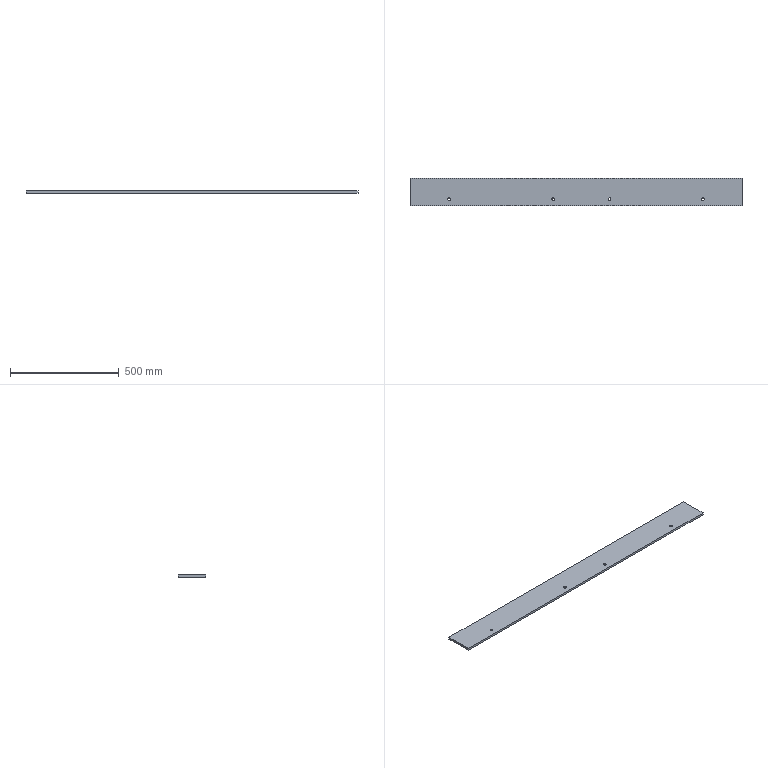Part | NX | features BREP 1 | 1 solid | 14 faces | box 1530 x 126 x 10 mm | volume 1923276 mm3 | cylinder 8 | plane 6 | commonest cylinder face diameters 12 x8
STEP:
#1=CARTESIAN_POINT('',(-591.,-33.,-5.));
#2=VERTEX_POINT('',#1);
#3=CARTESIAN_POINT('',(-579.,-33.,-5.));
#4=VERTEX_POINT('',#3);
#5=CARTESIAN_POINT('',(-585.,-33.,-5.));
#6=DIRECTION('',(0.,0.,-1.));
#7=DIRECTION('',(1.,0.,0.));
#8=AXIS2_PLACEMENT_3D('',#5,#6,#7);
#9=CIRCLE('',#8,6.);
#10=EDGE_CURVE('',#2,#4,#9,.T.);
#11=ORIENTED_EDGE('',*,*,#10,.T.);
#12=CARTESIAN_POINT('',(-579.,-33.,5.));
#13=VERTEX_POINT('',#12);
#14=CARTESIAN_POINT('',(-579.,-33.,-5.));
#15=DIRECTION('',(0.,0.,1.));
#16=VECTOR('',#15,1000.);
#17=LINE('',#14,#16);
#18=EDGE_CURVE('',#13,#4,#17,.F.);
#19=ORIENTED_EDGE('',*,*,#18,.F.);
#20=CARTESIAN_POINT('',(-591.,-33.,5.));
#21=VERTEX_POINT('',#20);
#22=CARTESIAN_POINT('',(-585.,-33.,5.));
#23=DIRECTION('',(0.,0.,-1.));
#24=DIRECTION('',(1.,0.,0.));
#25=AXIS2_PLACEMENT_3D('',#22,#23,#24);
#26=CIRCLE('',#25,6.);
#27=EDGE_CURVE('',#21,#13,#26,.T.);
#28=ORIENTED_EDGE('',*,*,#27,.F.);
#29=CARTESIAN_POINT('',(-591.,-33.,-5.));
#30=DIRECTION('',(0.,0.,1.));
#31=VECTOR('',#30,1000.);
#32=LINE('',#29,#31);
#33=EDGE_CURVE('',#21,#2,#32,.F.);
#34=ORIENTED_EDGE('',*,*,#33,.T.);
#35=EDGE_LOOP('',(#11,#19,#28,#34));
#36=FACE_BOUND('',#35,.T.);
#37=CARTESIAN_POINT('',(-585.,-33.,-5.));
#38=DIRECTION('',(0.,0.,1.));
#39=DIRECTION('',(1.,0.,0.));
#40=AXIS2_PLACEMENT_3D('',#37,#38,#39);
#41=CYLINDRICAL_SURFACE('',#40,6.);
#42=ADVANCED_FACE('',(#36),#41,.F.);
#43=CARTESIAN_POINT('',(-111.,-33.,-5.));
#44=VERTEX_POINT('',#43);
#45=CARTESIAN_POINT('',(-99.,-33.,-5.));
#46=VERTEX_POINT('',#45);
#47=CARTESIAN_POINT('',(-105.,-33.,-5.));
#48=DIRECTION('',(0.,0.,-1.));
#49=DIRECTION('',(1.,0.,0.));
#50=AXIS2_PLACEMENT_3D('',#47,#48,#49);
#51=CIRCLE('',#50,6.);
#52=EDGE_CURVE('',#44,#46,#51,.T.);
#53=ORIENTED_EDGE('',*,*,#52,.T.);
#54=CARTESIAN_POINT('',(-99.,-33.,5.));
#55=VERTEX_POINT('',#54);
#56=CARTESIAN_POINT('',(-99.,-33.,-5.));
#57=DIRECTION('',(0.,0.,1.));
#58=VECTOR('',#57,1000.);
#59=LINE('',#56,#58);
#60=EDGE_CURVE('',#55,#46,#59,.F.);
#61=ORIENTED_EDGE('',*,*,#60,.F.);
#62=CARTESIAN_POINT('',(-111.,-33.,5.));
#63=VERTEX_POINT('',#62);
#64=CARTESIAN_POINT('',(-105.,-33.,5.));
#65=DIRECTION('',(0.,0.,-1.));
#66=DIRECTION('',(1.,0.,0.));
#67=AXIS2_PLACEMENT_3D('',#64,#65,#66);
#68=CIRCLE('',#67,6.);
#69=EDGE_CURVE('',#63,#55,#68,.T.);
#70=ORIENTED_EDGE('',*,*,#69,.F.);
#71=CARTESIAN_POINT('',(-111.,-33.,-5.));
#72=DIRECTION('',(0.,0.,1.));
#73=VECTOR('',#72,1000.);
#74=LINE('',#71,#73);
#75=EDGE_CURVE('',#63,#44,#74,.F.);
#76=ORIENTED_EDGE('',*,*,#75,.T.);
#77=EDGE_LOOP('',(#53,#61,#70,#76));
#78=FACE_BOUND('',#77,.T.);
#79=CARTESIAN_POINT('',(-105.,-33.,-5.));
#80=DIRECTION('',(0.,0.,1.));
#81=DIRECTION('',(1.,0.,0.));
#82=AXIS2_PLACEMENT_3D('',#79,#80,#81);
#83=CYLINDRICAL_SURFACE('',#82,6.);
#84=ADVANCED_FACE('',(#78),#83,.F.);
#85=CARTESIAN_POINT('',(149.,-33.,-5.));
#86=VERTEX_POINT('',#85);
#87=CARTESIAN_POINT('',(161.,-33.,-5.));
#88=VERTEX_POINT('',#87);
#89=CARTESIAN_POINT('',(155.,-33.,-5.));
#90=DIRECTION('',(0.,0.,-1.));
#91=DIRECTION('',(-1.,0.,0.));
#92=AXIS2_PLACEMENT_3D('',#89,#90,#91);
#93=CIRCLE('',#92,6.);
#94=EDGE_CURVE('',#86,#88,#93,.T.);
#95=ORIENTED_EDGE('',*,*,#94,.T.);
#96=CARTESIAN_POINT('',(161.,-33.,5.));
#97=VERTEX_POINT('',#96);
#98=CARTESIAN_POINT('',(161.,-33.,-5.));
#99=DIRECTION('',(0.,0.,1.));
#100=VECTOR('',#99,1000.);
#101=LINE('',#98,#100);
#102=EDGE_CURVE('',#97,#88,#101,.F.);
#103=ORIENTED_EDGE('',*,*,#102,.F.);
#104=CARTESIAN_POINT('',(149.,-33.,5.));
#105=VERTEX_POINT('',#104);
#106=CARTESIAN_POINT('',(155.,-33.,5.));
#107=DIRECTION('',(0.,0.,-1.));
#108=DIRECTION('',(-1.,0.,0.));
#109=AXIS2_PLACEMENT_3D('',#106,#107,#108);
#110=CIRCLE('',#109,6.);
#111=EDGE_CURVE('',#105,#97,#110,.T.);
#112=ORIENTED_EDGE('',*,*,#111,.F.);
#113=CARTESIAN_POINT('',(149.,-33.,-5.));
#114=DIRECTION('',(0.,0.,1.));
#115=VECTOR('',#114,1000.);
#116=LINE('',#113,#115);
#117=EDGE_CURVE('',#105,#86,#116,.F.);
#118=ORIENTED_EDGE('',*,*,#117,.T.);
#119=EDGE_LOOP('',(#95,#103,#112,#118));
#120=FACE_BOUND('',#119,.T.);
#121=CARTESIAN_POINT('',(155.,-33.,-5.));
#122=DIRECTION('',(0.,0.,1.));
#123=DIRECTION('',(1.,0.,0.));
#124=AXIS2_PLACEMENT_3D('',#121,#122,#123);
#125=CYLINDRICAL_SURFACE('',#124,6.);
#126=ADVANCED_FACE('',(#120),#125,.F.);
#127=CARTESIAN_POINT('',(579.,-33.,-5.));
#128=VERTEX_POINT('',#127);
#129=CARTESIAN_POINT('',(591.,-33.,-5.));
#130=VERTEX_POINT('',#129);
#131=CARTESIAN_POINT('',(585.,-33.,-5.));
#132=DIRECTION('',(0.,0.,-1.));
#133=DIRECTION('',(-1.,0.,0.));
#134=AXIS2_PLACEMENT_3D('',#131,#132,#133);
#135=CIRCLE('',#134,6.);
#136=EDGE_CURVE('',#128,#130,#135,.T.);
#137=ORIENTED_EDGE('',*,*,#136,.T.);
#138=CARTESIAN_POINT('',(591.,-33.,5.));
#139=VERTEX_POINT('',#138);
#140=CARTESIAN_POINT('',(591.,-33.,-5.));
#141=DIRECTION('',(0.,0.,1.));
#142=VECTOR('',#141,1000.);
#143=LINE('',#140,#142);
#144=EDGE_CURVE('',#139,#130,#143,.F.);
#145=ORIENTED_EDGE('',*,*,#144,.F.);
#146=CARTESIAN_POINT('',(579.,-33.,5.));
#147=VERTEX_POINT('',#146);
#148=CARTESIAN_POINT('',(585.,-33.,5.));
#149=DIRECTION('',(0.,0.,-1.));
#150=DIRECTION('',(-1.,0.,0.));
#151=AXIS2_PLACEMENT_3D('',#148,#149,#150);
#152=CIRCLE('',#151,6.);
#153=EDGE_CURVE('',#147,#139,#152,.T.);
#154=ORIENTED_EDGE('',*,*,#153,.F.);
#155=CARTESIAN_POINT('',(579.,-33.,-5.));
#156=DIRECTION('',(0.,0.,1.));
#157=VECTOR('',#156,1000.);
#158=LINE('',#155,#157);
#159=EDGE_CURVE('',#147,#128,#158,.F.);
#160=ORIENTED_EDGE('',*,*,#159,.T.);
#161=EDGE_LOOP('',(#137,#145,#154,#160));
#162=FACE_BOUND('',#161,.T.);
#163=CARTESIAN_POINT('',(585.,-33.,-5.));
#164=DIRECTION('',(0.,0.,1.));
#165=DIRECTION('',(1.,0.,0.));
#166=AXIS2_PLACEMENT_3D('',#163,#164,#165);
#167=CYLINDRICAL_SURFACE('',#166,6.);
#168=ADVANCED_FACE('',(#162),#167,.F.);
#169=CARTESIAN_POINT('',(-765.,63.,5.));
#170=VERTEX_POINT('',#169);
#171=CARTESIAN_POINT('',(-765.,-63.,5.));
#172=VERTEX_POINT('',#171);
#173=CARTESIAN_POINT('',(-765.,63.,5.));
#174=DIRECTION('',(0.,-1.,0.));
#175=VECTOR('',#174,1000.);
#176=LINE('',#173,#175);
#177=EDGE_CURVE('',#170,#172,#176,.T.);
#178=ORIENTED_EDGE('',*,*,#177,.F.);
#179=CARTESIAN_POINT('',(-765.,63.,-5.));
#180=VERTEX_POINT('',#179);
#181=CARTESIAN_POINT('',(-765.,63.,-5.));
#182=DIRECTION('',(0.,0.,1.));
#183=VECTOR('',#182,1000.);
#184=LINE('',#181,#183);
#185=EDGE_CURVE('',#180,#170,#184,.T.);
#186=ORIENTED_EDGE('',*,*,#185,.F.);
#187=CARTESIAN_POINT('',(-765.,-63.,-5.));
#188=VERTEX_POINT('',#187);
#189=CARTESIAN_POINT('',(-765.,63.,-5.));
#190=DIRECTION('',(0.,-1.,0.));
#191=VECTOR('',#190,1000.);
#192=LINE('',#189,#191);
#193=EDGE_CURVE('',#180,#188,#192,.T.);
#194=ORIENTED_EDGE('',*,*,#193,.T.);
#195=CARTESIAN_POINT('',(-765.,-63.,-5.));
#196=DIRECTION('',(0.,0.,1.));
#197=VECTOR('',#196,1000.);
#198=LINE('',#195,#197);
#199=EDGE_CURVE('',#188,#172,#198,.T.);
#200=ORIENTED_EDGE('',*,*,#199,.T.);
#201=EDGE_LOOP('',(#178,#186,#194,#200));
#202=FACE_BOUND('',#201,.T.);
#203=CARTESIAN_POINT('',(-765.,63.,-5.));
#204=DIRECTION('',(1.,0.,0.));
#205=DIRECTION('',(0.,0.,-1.));
#206=AXIS2_PLACEMENT_3D('',#203,#204,#205);
#207=PLANE('',#206);
#208=ADVANCED_FACE('',(#202),#207,.F.);
#209=CARTESIAN_POINT('',(765.,-63.,5.));
#210=VERTEX_POINT('',#209);
#211=CARTESIAN_POINT('',(-765.,-63.,5.));
#212=DIRECTION('',(1.,0.,0.));
#213=VECTOR('',#212,1000.);
#214=LINE('',#211,#213);
#215=EDGE_CURVE('',#172,#210,#214,.T.);
#216=ORIENTED_EDGE('',*,*,#215,.F.);
#217=ORIENTED_EDGE('',*,*,#199,.F.);
#218=CARTESIAN_POINT('',(765.,-63.,-5.));
#219=VERTEX_POINT('',#218);
#220=CARTESIAN_POINT('',(-765.,-63.,-5.));
#221=DIRECTION('',(1.,0.,0.));
#222=VECTOR('',#221,1000.);
#223=LINE('',#220,#222);
#224=EDGE_CURVE('',#188,#219,#223,.T.);
#225=ORIENTED_EDGE('',*,*,#224,.T.);
#226=CARTESIAN_POINT('',(765.,-63.,-5.));
#227=DIRECTION('',(0.,0.,1.));
#228=VECTOR('',#227,1000.);
#229=LINE('',#226,#228);
#230=EDGE_CURVE('',#219,#210,#229,.T.);
#231=ORIENTED_EDGE('',*,*,#230,.T.);
#232=EDGE_LOOP('',(#216,#217,#225,#231));
#233=FACE_BOUND('',#232,.T.);
#234=CARTESIAN_POINT('',(-765.,-63.,-5.));
#235=DIRECTION('',(0.,1.,0.));
#236=DIRECTION('',(0.,0.,1.));
#237=AXIS2_PLACEMENT_3D('',#234,#235,#236);
#238=PLANE('',#237);
#239=ADVANCED_FACE('',(#233),#238,.F.);
#240=CARTESIAN_POINT('',(765.,63.,5.));
#241=VERTEX_POINT('',#240);
#242=CARTESIAN_POINT('',(765.,63.,5.));
#243=DIRECTION('',(0.,1.,0.));
#244=VECTOR('',#243,1000.);
#245=LINE('',#242,#244);
#246=EDGE_CURVE('',#210,#241,#245,.T.);
#247=ORIENTED_EDGE('',*,*,#246,.F.);
#248=ORIENTED_EDGE('',*,*,#230,.F.);
#249=CARTESIAN_POINT('',(765.,63.,-5.));
#250=VERTEX_POINT('',#249);
#251=CARTESIAN_POINT('',(765.,63.,-5.));
#252=DIRECTION('',(0.,1.,0.));
#253=VECTOR('',#252,1000.);
#254=LINE('',#251,#253);
#255=EDGE_CURVE('',#219,#250,#254,.T.);
#256=ORIENTED_EDGE('',*,*,#255,.T.);
#257=CARTESIAN_POINT('',(765.,63.,-5.));
#258=DIRECTION('',(0.,0.,1.));
#259=VECTOR('',#258,1000.);
#260=LINE('',#257,#259);
#261=EDGE_CURVE('',#250,#241,#260,.T.);
#262=ORIENTED_EDGE('',*,*,#261,.T.);
#263=EDGE_LOOP('',(#247,#248,#256,#262));
#264=FACE_BOUND('',#263,.T.);
#265=CARTESIAN_POINT('',(765.,63.,-5.));
#266=DIRECTION('',(-1.,0.,0.));
#267=DIRECTION('',(0.,0.,1.));
#268=AXIS2_PLACEMENT_3D('',#265,#266,#267);
#269=PLANE('',#268);
#270=ADVANCED_FACE('',(#264),#269,.F.);
#271=CARTESIAN_POINT('',(-765.,63.,5.));
#272=DIRECTION('',(-1.,0.,0.));
#273=VECTOR('',#272,1000.);
#274=LINE('',#271,#273);
#275=EDGE_CURVE('',#241,#170,#274,.T.);
#276=ORIENTED_EDGE('',*,*,#275,.F.);
#277=ORIENTED_EDGE('',*,*,#261,.F.);
#278=CARTESIAN_POINT('',(-765.,63.,-5.));
#279=DIRECTION('',(-1.,0.,0.));
#280=VECTOR('',#279,1000.);
#281=LINE('',#278,#280);
#282=EDGE_CURVE('',#250,#180,#281,.T.);
#283=ORIENTED_EDGE('',*,*,#282,.T.);
#284=ORIENTED_EDGE('',*,*,#185,.T.);
#285=EDGE_LOOP('',(#276,#277,#283,#284));
#286=FACE_BOUND('',#285,.T.);
#287=CARTESIAN_POINT('',(-765.,63.,-5.));
#288=DIRECTION('',(0.,-1.,0.));
#289=DIRECTION('',(0.,0.,-1.));
#290=AXIS2_PLACEMENT_3D('',#287,#288,#289);
#291=PLANE('',#290);
#292=ADVANCED_FACE('',(#286),#291,.F.);
#293=ORIENTED_EDGE('',*,*,#10,.F.);
#294=CARTESIAN_POINT('',(-585.,-33.,-5.));
#295=DIRECTION('',(0.,0.,-1.));
#296=DIRECTION('',(1.,0.,0.));
#297=AXIS2_PLACEMENT_3D('',#294,#295,#296);
#298=CIRCLE('',#297,6.);
#299=EDGE_CURVE('',#4,#2,#298,.T.);
#300=ORIENTED_EDGE('',*,*,#299,.F.);
#301=EDGE_LOOP('',(#293,#300));
#302=FACE_BOUND('',#301,.T.);
#303=ORIENTED_EDGE('',*,*,#52,.F.);
#304=CARTESIAN_POINT('',(-105.,-33.,-5.));
#305=DIRECTION('',(0.,0.,-1.));
#306=DIRECTION('',(1.,0.,0.));
#307=AXIS2_PLACEMENT_3D('',#304,#305,#306);
#308=CIRCLE('',#307,6.);
#309=EDGE_CURVE('',#46,#44,#308,.T.);
#310=ORIENTED_EDGE('',*,*,#309,.F.);
#311=EDGE_LOOP('',(#303,#310));
#312=FACE_BOUND('',#311,.T.);
#313=ORIENTED_EDGE('',*,*,#94,.F.);
#314=CARTESIAN_POINT('',(155.,-33.,-5.));
#315=DIRECTION('',(0.,0.,-1.));
#316=DIRECTION('',(-1.,0.,0.));
#317=AXIS2_PLACEMENT_3D('',#314,#315,#316);
#318=CIRCLE('',#317,6.);
#319=EDGE_CURVE('',#88,#86,#318,.T.);
#320=ORIENTED_EDGE('',*,*,#319,.F.);
#321=EDGE_LOOP('',(#313,#320));
#322=FACE_BOUND('',#321,.T.);
#323=ORIENTED_EDGE('',*,*,#136,.F.);
#324=CARTESIAN_POINT('',(585.,-33.,-5.));
#325=DIRECTION('',(0.,0.,-1.));
#326=DIRECTION('',(-1.,0.,0.));
#327=AXIS2_PLACEMENT_3D('',#324,#325,#326);
#328=CIRCLE('',#327,6.);
#329=EDGE_CURVE('',#130,#128,#328,.T.);
#330=ORIENTED_EDGE('',*,*,#329,.F.);
#331=EDGE_LOOP('',(#323,#330));
#332=FACE_BOUND('',#331,.T.);
#333=ORIENTED_EDGE('',*,*,#193,.F.);
#334=ORIENTED_EDGE('',*,*,#282,.F.);
#335=ORIENTED_EDGE('',*,*,#255,.F.);
#336=ORIENTED_EDGE('',*,*,#224,.F.);
#337=EDGE_LOOP('',(#333,#334,#335,#336));
#338=FACE_BOUND('',#337,.T.);
#339=CARTESIAN_POINT('',(-765.,-63.,-5.));
#340=DIRECTION('',(0.,0.,-1.));
#341=DIRECTION('',(-1.,0.,0.));
#342=AXIS2_PLACEMENT_3D('',#339,#340,#341);
#343=PLANE('',#342);
#344=ADVANCED_FACE('',(#302,#312,#322,#332,#338),#343,.T.);
#345=ORIENTED_EDGE('',*,*,#27,.T.);
#346=CARTESIAN_POINT('',(-585.,-33.,5.));
#347=DIRECTION('',(0.,0.,-1.));
#348=DIRECTION('',(1.,0.,0.));
#349=AXIS2_PLACEMENT_3D('',#346,#347,#348);
#350=CIRCLE('',#349,6.);
#351=EDGE_CURVE('',#13,#21,#350,.T.);
#352=ORIENTED_EDGE('',*,*,#351,.T.);
#353=EDGE_LOOP('',(#345,#352));
#354=FACE_BOUND('',#353,.T.);
#355=ORIENTED_EDGE('',*,*,#69,.T.);
#356=CARTESIAN_POINT('',(-105.,-33.,5.));
#357=DIRECTION('',(0.,0.,-1.));
#358=DIRECTION('',(1.,0.,0.));
#359=AXIS2_PLACEMENT_3D('',#356,#357,#358);
#360=CIRCLE('',#359,6.);
#361=EDGE_CURVE('',#55,#63,#360,.T.);
#362=ORIENTED_EDGE('',*,*,#361,.T.);
#363=EDGE_LOOP('',(#355,#362));
#364=FACE_BOUND('',#363,.T.);
#365=ORIENTED_EDGE('',*,*,#111,.T.);
#366=CARTESIAN_POINT('',(155.,-33.,5.));
#367=DIRECTION('',(0.,0.,-1.));
#368=DIRECTION('',(-1.,0.,0.));
#369=AXIS2_PLACEMENT_3D('',#366,#367,#368);
#370=CIRCLE('',#369,6.);
#371=EDGE_CURVE('',#97,#105,#370,.T.);
#372=ORIENTED_EDGE('',*,*,#371,.T.);
#373=EDGE_LOOP('',(#365,#372));
#374=FACE_BOUND('',#373,.T.);
#375=ORIENTED_EDGE('',*,*,#153,.T.);
#376=CARTESIAN_POINT('',(585.,-33.,5.));
#377=DIRECTION('',(0.,0.,-1.));
#378=DIRECTION('',(-1.,0.,0.));
#379=AXIS2_PLACEMENT_3D('',#376,#377,#378);
#380=CIRCLE('',#379,6.);
#381=EDGE_CURVE('',#139,#147,#380,.T.);
#382=ORIENTED_EDGE('',*,*,#381,.T.);
#383=EDGE_LOOP('',(#375,#382));
#384=FACE_BOUND('',#383,.T.);
#385=ORIENTED_EDGE('',*,*,#177,.T.);
#386=ORIENTED_EDGE('',*,*,#215,.T.);
#387=ORIENTED_EDGE('',*,*,#246,.T.);
#388=ORIENTED_EDGE('',*,*,#275,.T.);
#389=EDGE_LOOP('',(#385,#386,#387,#388));
#390=FACE_BOUND('',#389,.T.);
#391=CARTESIAN_POINT('',(-765.,-63.,5.));
#392=DIRECTION('',(0.,0.,-1.));
#393=DIRECTION('',(-1.,0.,0.));
#394=AXIS2_PLACEMENT_3D('',#391,#392,#393);
#395=PLANE('',#394);
#396=ADVANCED_FACE('',(#354,#364,#374,#384,#390),#395,.F.);
#397=ORIENTED_EDGE('',*,*,#144,.T.);
#398=ORIENTED_EDGE('',*,*,#329,.T.);
#399=ORIENTED_EDGE('',*,*,#159,.F.);
#400=ORIENTED_EDGE('',*,*,#381,.F.);
#401=EDGE_LOOP('',(#397,#398,#399,#400));
#402=FACE_BOUND('',#401,.T.);
#403=CARTESIAN_POINT('',(585.,-33.,-5.));
#404=DIRECTION('',(0.,0.,1.));
#405=DIRECTION('',(1.,0.,0.));
#406=AXIS2_PLACEMENT_3D('',#403,#404,#405);
#407=CYLINDRICAL_SURFACE('',#406,6.);
#408=ADVANCED_FACE('',(#402),#407,.F.);
#409=ORIENTED_EDGE('',*,*,#102,.T.);
#410=ORIENTED_EDGE('',*,*,#319,.T.);
#411=ORIENTED_EDGE('',*,*,#117,.F.);
#412=ORIENTED_EDGE('',*,*,#371,.F.);
#413=EDGE_LOOP('',(#409,#410,#411,#412));
#414=FACE_BOUND('',#413,.T.);
#415=CARTESIAN_POINT('',(155.,-33.,-5.));
#416=DIRECTION('',(0.,0.,1.));
#417=DIRECTION('',(1.,0.,0.));
#418=AXIS2_PLACEMENT_3D('',#415,#416,#417);
#419=CYLINDRICAL_SURFACE('',#418,6.);
#420=ADVANCED_FACE('',(#414),#419,.F.);
#421=ORIENTED_EDGE('',*,*,#60,.T.);
#422=ORIENTED_EDGE('',*,*,#309,.T.);
#423=ORIENTED_EDGE('',*,*,#75,.F.);
#424=ORIENTED_EDGE('',*,*,#361,.F.);
#425=EDGE_LOOP('',(#421,#422,#423,#424));
#426=FACE_BOUND('',#425,.T.);
#427=CARTESIAN_POINT('',(-105.,-33.,-5.));
#428=DIRECTION('',(0.,0.,1.));
#429=DIRECTION('',(1.,0.,0.));
#430=AXIS2_PLACEMENT_3D('',#427,#428,#429);
#431=CYLINDRICAL_SURFACE('',#430,6.);
#432=ADVANCED_FACE('',(#426),#431,.F.);
#433=ORIENTED_EDGE('',*,*,#18,.T.);
#434=ORIENTED_EDGE('',*,*,#299,.T.);
#435=ORIENTED_EDGE('',*,*,#33,.F.);
#436=ORIENTED_EDGE('',*,*,#351,.F.);
#437=EDGE_LOOP('',(#433,#434,#435,#436));
#438=FACE_BOUND('',#437,.T.);
#439=CARTESIAN_POINT('',(-585.,-33.,-5.));
#440=DIRECTION('',(0.,0.,1.));
#441=DIRECTION('',(1.,0.,0.));
#442=AXIS2_PLACEMENT_3D('',#439,#440,#441);
#443=CYLINDRICAL_SURFACE('',#442,6.);
#444=ADVANCED_FACE('',(#438),#443,.F.);
#445=CLOSED_SHELL('',(#42,#84,#126,#168,#208,#239,#270,#292,#344,#396,#408,#420,#432,#444));
#446=MANIFOLD_SOLID_BREP('',#445);
#447=(LENGTH_UNIT()NAMED_UNIT(*)SI_UNIT(.MILLI.,.METRE.));
#448=UNCERTAINTY_MEASURE_WITH_UNIT(LENGTH_MEASURE(0.00001),#447,'','');
#449=(NAMED_UNIT(*)PLANE_ANGLE_UNIT()SI_UNIT($,.RADIAN.));
#450=(NAMED_UNIT(*)SI_UNIT($,.STERADIAN.)SOLID_ANGLE_UNIT());
#451=(GEOMETRIC_REPRESENTATION_CONTEXT(3)GLOBAL_UNCERTAINTY_ASSIGNED_CONTEXT((#448))GLOBAL_UNIT_ASSIGNED_CONTEXT((#447,#449,#450))REPRESENTATION_CONTEXT('',''));
#452=ADVANCED_BREP_SHAPE_REPRESENTATION('',(#446),#451);